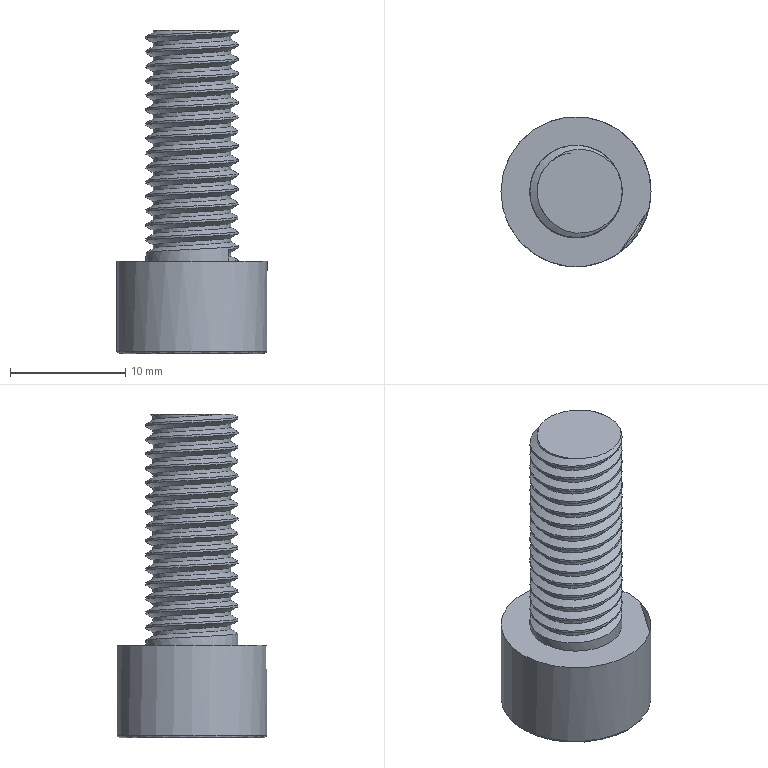Part | STEP file | Tube feed_id190_x_t | 1 solid | 24 faces | box 13 x 13 x 28 mm | volume 1756 mm3 | plane 11 | cylinder 9 | spline 3 | torus 1 | commonest cylinder face diameters 0.4 x6 6.75 x1 8 x1 13 x1